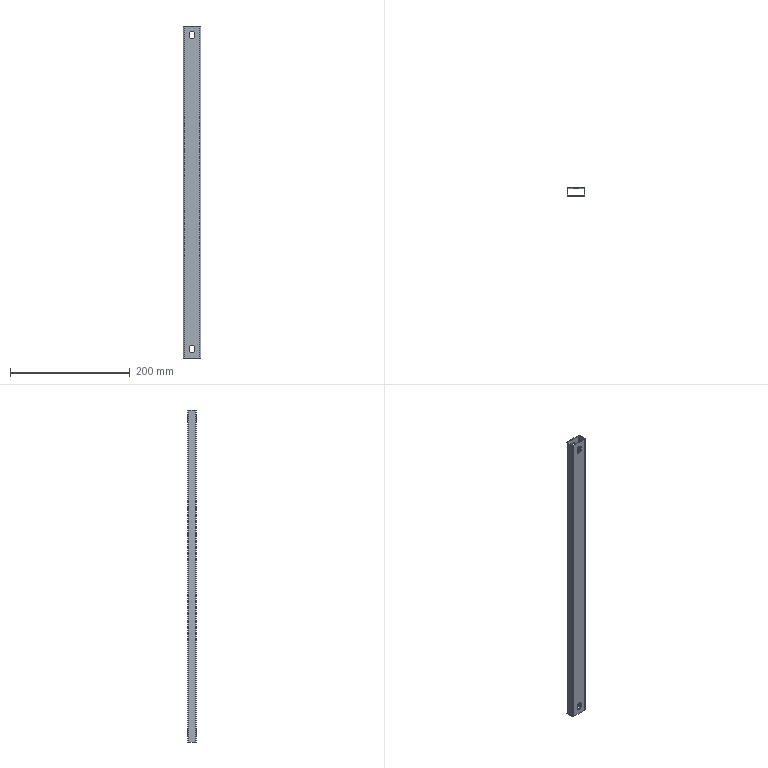Part | STEP file | 7100901 | 1 solid | 34 faces | box 30 x 15 x 555 mm | volume 54621 mm3 | plane 18 | cylinder 16 | commonest cylinder face diameters 10 x8 1.6 x4 4 x4